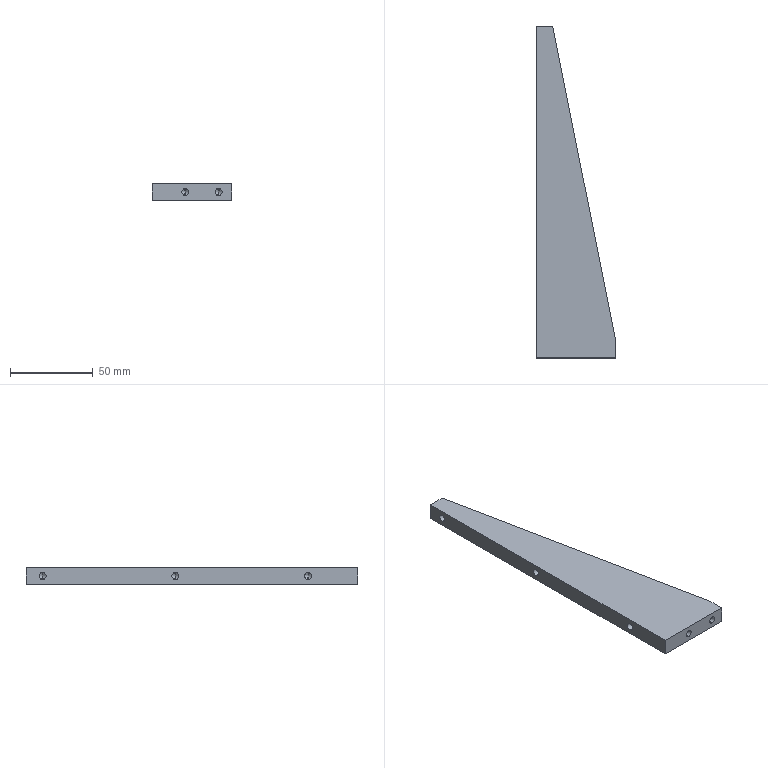Part | STEP file | PN_0046 Mount electronic clip reinforcing rib A | 1 solid | 27 faces | box 48 x 200 x 10 mm | volume 59178 mm3 | cylinder 10 | cone 10 | plane 7 | commonest cylinder face diameters 4.2 x10